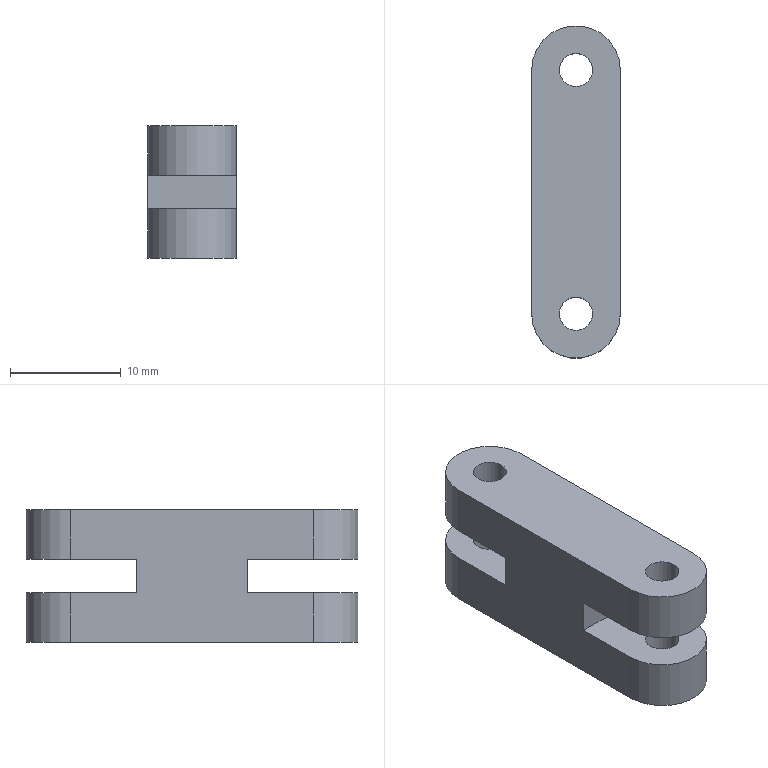Part | SolidWorks | features ICE 2, 3DProfileFeature 1, Extrusion 1, HoleWzd 1 | 1 solid | 26 faces | box 8 x 30 x 12 mm | volume 2022 mm3 | cylinder 14 | plane 10 | cone 2 | commonest cylinder face diameters 3 x8 8 x4 5 x2
STEP:
#1=CARTESIAN_POINT('',(-2.,11.,8.5));
#2=VERTEX_POINT('',#1);
#3=CARTESIAN_POINT('',(-2.,11.,3.5));
#4=VERTEX_POINT('',#3);
#5=CARTESIAN_POINT('',(-2.,11.,6.));
#6=DIRECTION('',(1.,0.,0.));
#7=DIRECTION('',(0.,0.,-1.));
#8=AXIS2_PLACEMENT_3D('',#5,#6,#7);
#9=CIRCLE('',#8,2.5);
#10=EDGE_CURVE('',#2,#4,#9,.T.);
#11=ORIENTED_EDGE('',*,*,#10,.F.);
#12=CARTESIAN_POINT('',(4.,11.,8.5));
#13=VERTEX_POINT('',#12);
#14=CARTESIAN_POINT('',(4.,11.,8.5));
#15=DIRECTION('',(1.,0.,0.));
#16=VECTOR('',#15,1000.);
#17=LINE('',#14,#16);
#18=EDGE_CURVE('',#2,#13,#17,.T.);
#19=ORIENTED_EDGE('',*,*,#18,.T.);
#20=CARTESIAN_POINT('',(4.,11.,3.5));
#21=VERTEX_POINT('',#20);
#22=CARTESIAN_POINT('',(4.,11.,6.));
#23=DIRECTION('',(1.,0.,0.));
#24=DIRECTION('',(0.,0.,-1.));
#25=AXIS2_PLACEMENT_3D('',#22,#23,#24);
#26=CIRCLE('',#25,2.5);
#27=EDGE_CURVE('',#13,#21,#26,.T.);
#28=ORIENTED_EDGE('',*,*,#27,.T.);
#29=CARTESIAN_POINT('',(4.,11.,3.5));
#30=DIRECTION('',(1.,0.,0.));
#31=VECTOR('',#30,1000.);
#32=LINE('',#29,#31);
#33=EDGE_CURVE('',#4,#21,#32,.T.);
#34=ORIENTED_EDGE('',*,*,#33,.F.);
#35=EDGE_LOOP('',(#11,#19,#28,#34));
#36=FACE_OUTER_BOUND('',#35,.T.);
#37=CARTESIAN_POINT('',(4.,11.,6.));
#38=DIRECTION('',(1.,0.,0.));
#39=DIRECTION('',(0.,0.,-1.));
#40=AXIS2_PLACEMENT_3D('',#37,#38,#39);
#41=CYLINDRICAL_SURFACE('',#40,2.5);
#42=ADVANCED_FACE('',(#36),#41,.F.);
#43=CARTESIAN_POINT('',(-3.502,11.,6.));
#44=VERTEX_POINT('',#43);
#45=CARTESIAN_POINT('',(-2.,11.,3.5));
#46=DIRECTION('',(0.515,0.,-0.8572));
#47=VECTOR('',#46,1000.);
#48=LINE('',#45,#47);
#49=EDGE_CURVE('',#44,#4,#48,.T.);
#50=ORIENTED_EDGE('',*,*,#49,.F.);
#51=CARTESIAN_POINT('',(-2.,11.,8.5));
#52=DIRECTION('',(0.515,0.,0.8572));
#53=VECTOR('',#52,1000.);
#54=LINE('',#51,#53);
#55=EDGE_CURVE('',#44,#2,#54,.T.);
#56=ORIENTED_EDGE('',*,*,#55,.T.);
#57=ORIENTED_EDGE('',*,*,#10,.T.);
#58=EDGE_LOOP('',(#50,#56,#57));
#59=FACE_OUTER_BOUND('',#58,.T.);
#60=CARTESIAN_POINT('',(-2.,11.,6.));
#61=DIRECTION('',(1.,0.,0.));
#62=DIRECTION('',(0.,0.,-1.));
#63=AXIS2_PLACEMENT_3D('',#60,#61,#62);
#64=CONICAL_SURFACE('',#63,2.5,1.03);
#65=ADVANCED_FACE('',(#59),#64,.F.);
#66=CARTESIAN_POINT('',(-1.5,0.,0.));
#67=VERTEX_POINT('',#66);
#68=CARTESIAN_POINT('',(1.5,0.,0.));
#69=VERTEX_POINT('',#68);
#70=CARTESIAN_POINT('',(0.,0.,0.));
#71=DIRECTION('',(0.,0.,1.));
#72=DIRECTION('',(1.,0.,0.));
#73=AXIS2_PLACEMENT_3D('',#70,#71,#72);
#74=CIRCLE('',#73,1.5);
#75=EDGE_CURVE('',#67,#69,#74,.T.);
#76=ORIENTED_EDGE('',*,*,#75,.F.);
#77=CARTESIAN_POINT('',(-1.5,0.,4.5));
#78=VERTEX_POINT('',#77);
#79=CARTESIAN_POINT('',(-1.5,0.,0.));
#80=DIRECTION('',(0.,0.,1.));
#81=VECTOR('',#80,1000.);
#82=LINE('',#79,#81);
#83=EDGE_CURVE('',#67,#78,#82,.T.);
#84=ORIENTED_EDGE('',*,*,#83,.T.);
#85=CARTESIAN_POINT('',(1.5,0.,4.5));
#86=VERTEX_POINT('',#85);
#87=CARTESIAN_POINT('',(0.,0.,4.5));
#88=DIRECTION('',(0.,0.,-1.));
#89=DIRECTION('',(-1.,0.,0.));
#90=AXIS2_PLACEMENT_3D('',#87,#88,#89);
#91=CIRCLE('',#90,1.5);
#92=EDGE_CURVE('',#86,#78,#91,.T.);
#93=ORIENTED_EDGE('',*,*,#92,.F.);
#94=CARTESIAN_POINT('',(1.5,0.,0.));
#95=DIRECTION('',(0.,0.,1.));
#96=VECTOR('',#95,1000.);
#97=LINE('',#94,#96);
#98=EDGE_CURVE('',#69,#86,#97,.T.);
#99=ORIENTED_EDGE('',*,*,#98,.F.);
#100=EDGE_LOOP('',(#76,#84,#93,#99));
#101=FACE_OUTER_BOUND('',#100,.T.);
#102=CARTESIAN_POINT('',(0.,0.,0.));
#103=DIRECTION('',(0.,0.,1.));
#104=DIRECTION('',(1.,0.,0.));
#105=AXIS2_PLACEMENT_3D('',#102,#103,#104);
#106=CYLINDRICAL_SURFACE('',#105,1.5);
#107=ADVANCED_FACE('',(#101),#106,.F.);
#108=CARTESIAN_POINT('',(-1.5,0.,7.5));
#109=VERTEX_POINT('',#108);
#110=CARTESIAN_POINT('',(1.5,0.,7.5));
#111=VERTEX_POINT('',#110);
#112=CARTESIAN_POINT('',(0.,0.,7.5));
#113=DIRECTION('',(0.,0.,1.));
#114=DIRECTION('',(0.,-1.,0.));
#115=AXIS2_PLACEMENT_3D('',#112,#113,#114);
#116=CIRCLE('',#115,1.5);
#117=EDGE_CURVE('',#109,#111,#116,.T.);
#118=ORIENTED_EDGE('',*,*,#117,.F.);
#119=CARTESIAN_POINT('',(-1.5,0.,12.));
#120=VERTEX_POINT('',#119);
#121=CARTESIAN_POINT('',(-1.5,0.,0.));
#122=DIRECTION('',(0.,0.,1.));
#123=VECTOR('',#122,1000.);
#124=LINE('',#121,#123);
#125=EDGE_CURVE('',#109,#120,#124,.T.);
#126=ORIENTED_EDGE('',*,*,#125,.T.);
#127=CARTESIAN_POINT('',(1.5,0.,12.));
#128=VERTEX_POINT('',#127);
#129=CARTESIAN_POINT('',(0.,0.,12.));
#130=DIRECTION('',(0.,0.,1.));
#131=DIRECTION('',(1.,0.,0.));
#132=AXIS2_PLACEMENT_3D('',#129,#130,#131);
#133=CIRCLE('',#132,1.5);
#134=EDGE_CURVE('',#120,#128,#133,.T.);
#135=ORIENTED_EDGE('',*,*,#134,.T.);
#136=CARTESIAN_POINT('',(1.5,0.,0.));
#137=DIRECTION('',(0.,0.,1.));
#138=VECTOR('',#137,1000.);
#139=LINE('',#136,#138);
#140=EDGE_CURVE('',#111,#128,#139,.T.);
#141=ORIENTED_EDGE('',*,*,#140,.F.);
#142=EDGE_LOOP('',(#118,#126,#135,#141));
#143=FACE_OUTER_BOUND('',#142,.T.);
#144=CARTESIAN_POINT('',(0.,0.,0.));
#145=DIRECTION('',(0.,0.,1.));
#146=DIRECTION('',(1.,0.,0.));
#147=AXIS2_PLACEMENT_3D('',#144,#145,#146);
#148=CYLINDRICAL_SURFACE('',#147,1.5);
#149=ADVANCED_FACE('',(#143),#148,.F.);
#150=CARTESIAN_POINT('',(-1.5,22.,7.5));
#151=VERTEX_POINT('',#150);
#152=CARTESIAN_POINT('',(1.5,22.,7.5));
#153=VERTEX_POINT('',#152);
#154=CARTESIAN_POINT('',(0.,22.,7.5));
#155=DIRECTION('',(0.,0.,1.));
#156=DIRECTION('',(0.,-1.,0.));
#157=AXIS2_PLACEMENT_3D('',#154,#155,#156);
#158=CIRCLE('',#157,1.5);
#159=EDGE_CURVE('',#151,#153,#158,.T.);
#160=ORIENTED_EDGE('',*,*,#159,.F.);
#161=CARTESIAN_POINT('',(-1.5,22.,12.));
#162=VERTEX_POINT('',#161);
#163=CARTESIAN_POINT('',(-1.5,22.,0.));
#164=DIRECTION('',(0.,0.,1.));
#165=VECTOR('',#164,1000.);
#166=LINE('',#163,#165);
#167=EDGE_CURVE('',#151,#162,#166,.T.);
#168=ORIENTED_EDGE('',*,*,#167,.T.);
#169=CARTESIAN_POINT('',(1.5,22.,12.));
#170=VERTEX_POINT('',#169);
#171=CARTESIAN_POINT('',(0.,22.,12.));
#172=DIRECTION('',(0.,0.,1.));
#173=DIRECTION('',(1.,0.,0.));
#174=AXIS2_PLACEMENT_3D('',#171,#172,#173);
#175=CIRCLE('',#174,1.5);
#176=EDGE_CURVE('',#162,#170,#175,.T.);
#177=ORIENTED_EDGE('',*,*,#176,.T.);
#178=CARTESIAN_POINT('',(1.5,22.,0.));
#179=DIRECTION('',(0.,0.,1.));
#180=VECTOR('',#179,1000.);
#181=LINE('',#178,#180);
#182=EDGE_CURVE('',#153,#170,#181,.T.);
#183=ORIENTED_EDGE('',*,*,#182,.F.);
#184=EDGE_LOOP('',(#160,#168,#177,#183));
#185=FACE_OUTER_BOUND('',#184,.T.);
#186=CARTESIAN_POINT('',(0.,22.,0.));
#187=DIRECTION('',(0.,0.,1.));
#188=DIRECTION('',(1.,0.,0.));
#189=AXIS2_PLACEMENT_3D('',#186,#187,#188);
#190=CYLINDRICAL_SURFACE('',#189,1.5);
#191=ADVANCED_FACE('',(#185),#190,.F.);
#192=CARTESIAN_POINT('',(-1.5,22.,0.));
#193=VERTEX_POINT('',#192);
#194=CARTESIAN_POINT('',(1.5,22.,0.));
#195=VERTEX_POINT('',#194);
#196=CARTESIAN_POINT('',(0.,22.,0.));
#197=DIRECTION('',(0.,0.,1.));
#198=DIRECTION('',(1.,0.,0.));
#199=AXIS2_PLACEMENT_3D('',#196,#197,#198);
#200=CIRCLE('',#199,1.5);
#201=EDGE_CURVE('',#193,#195,#200,.T.);
#202=ORIENTED_EDGE('',*,*,#201,.F.);
#203=CARTESIAN_POINT('',(-1.5,22.,4.5));
#204=VERTEX_POINT('',#203);
#205=CARTESIAN_POINT('',(-1.5,22.,0.));
#206=DIRECTION('',(0.,0.,1.));
#207=VECTOR('',#206,1000.);
#208=LINE('',#205,#207);
#209=EDGE_CURVE('',#193,#204,#208,.T.);
#210=ORIENTED_EDGE('',*,*,#209,.T.);
#211=CARTESIAN_POINT('',(1.5,22.,4.5));
#212=VERTEX_POINT('',#211);
#213=CARTESIAN_POINT('',(0.,22.,4.5));
#214=DIRECTION('',(0.,0.,-1.));
#215=DIRECTION('',(-1.,0.,0.));
#216=AXIS2_PLACEMENT_3D('',#213,#214,#215);
#217=CIRCLE('',#216,1.5);
#218=EDGE_CURVE('',#212,#204,#217,.T.);
#219=ORIENTED_EDGE('',*,*,#218,.F.);
#220=CARTESIAN_POINT('',(1.5,22.,0.));
#221=DIRECTION('',(0.,0.,1.));
#222=VECTOR('',#221,1000.);
#223=LINE('',#220,#222);
#224=EDGE_CURVE('',#195,#212,#223,.T.);
#225=ORIENTED_EDGE('',*,*,#224,.F.);
#226=EDGE_LOOP('',(#202,#210,#219,#225));
#227=FACE_OUTER_BOUND('',#226,.T.);
#228=CARTESIAN_POINT('',(0.,22.,0.));
#229=DIRECTION('',(0.,0.,1.));
#230=DIRECTION('',(1.,0.,0.));
#231=AXIS2_PLACEMENT_3D('',#228,#229,#230);
#232=CYLINDRICAL_SURFACE('',#231,1.5);
#233=ADVANCED_FACE('',(#227),#232,.F.);
#234=CARTESIAN_POINT('',(4.,0.,4.5));
#235=VERTEX_POINT('',#234);
#236=CARTESIAN_POINT('',(4.,0.,0.));
#237=VERTEX_POINT('',#236);
#238=CARTESIAN_POINT('',(4.,0.,12.));
#239=DIRECTION('',(0.,0.,-1.));
#240=VECTOR('',#239,1000.);
#241=LINE('',#238,#240);
#242=EDGE_CURVE('',#235,#237,#241,.T.);
#243=ORIENTED_EDGE('',*,*,#242,.F.);
#244=CARTESIAN_POINT('',(-4.,0.,4.5));
#245=VERTEX_POINT('',#244);
#246=CARTESIAN_POINT('',(0.,0.,4.5));
#247=DIRECTION('',(0.,0.,-1.));
#248=DIRECTION('',(-1.,0.,0.));
#249=AXIS2_PLACEMENT_3D('',#246,#247,#248);
#250=CIRCLE('',#249,4.);
#251=EDGE_CURVE('',#235,#245,#250,.T.);
#252=ORIENTED_EDGE('',*,*,#251,.T.);
#253=CARTESIAN_POINT('',(-4.,0.,0.));
#254=VERTEX_POINT('',#253);
#255=CARTESIAN_POINT('',(-4.,0.,12.));
#256=DIRECTION('',(0.,0.,-1.));
#257=VECTOR('',#256,1000.);
#258=LINE('',#255,#257);
#259=EDGE_CURVE('',#245,#254,#258,.T.);
#260=ORIENTED_EDGE('',*,*,#259,.T.);
#261=CARTESIAN_POINT('',(0.,0.,0.));
#262=DIRECTION('',(0.,0.,1.));
#263=DIRECTION('',(1.,0.,0.));
#264=AXIS2_PLACEMENT_3D('',#261,#262,#263);
#265=CIRCLE('',#264,4.);
#266=EDGE_CURVE('',#254,#237,#265,.T.);
#267=ORIENTED_EDGE('',*,*,#266,.T.);
#268=EDGE_LOOP('',(#243,#252,#260,#267));
#269=FACE_OUTER_BOUND('',#268,.T.);
#270=CARTESIAN_POINT('',(0.,0.,12.));
#271=DIRECTION('',(0.,0.,-1.));
#272=DIRECTION('',(-1.,0.,0.));
#273=AXIS2_PLACEMENT_3D('',#270,#271,#272);
#274=CYLINDRICAL_SURFACE('',#273,4.);
#275=ADVANCED_FACE('',(#269),#274,.T.);
#276=CARTESIAN_POINT('',(4.,22.,12.));
#277=VERTEX_POINT('',#276);
#278=CARTESIAN_POINT('',(4.,22.,7.5));
#279=VERTEX_POINT('',#278);
#280=CARTESIAN_POINT('',(4.,22.,12.));
#281=DIRECTION('',(0.,0.,-1.));
#282=VECTOR('',#281,1000.);
#283=LINE('',#280,#282);
#284=EDGE_CURVE('',#277,#279,#283,.T.);
#285=ORIENTED_EDGE('',*,*,#284,.T.);
#286=CARTESIAN_POINT('',(-4.,22.,7.5));
#287=VERTEX_POINT('',#286);
#288=CARTESIAN_POINT('',(0.,22.,7.5));
#289=DIRECTION('',(0.,0.,1.));
#290=DIRECTION('',(0.,-1.,0.));
#291=AXIS2_PLACEMENT_3D('',#288,#289,#290);
#292=CIRCLE('',#291,4.);
#293=EDGE_CURVE('',#279,#287,#292,.T.);
#294=ORIENTED_EDGE('',*,*,#293,.T.);
#295=CARTESIAN_POINT('',(-4.,22.,12.));
#296=VERTEX_POINT('',#295);
#297=CARTESIAN_POINT('',(-4.,22.,12.));
#298=DIRECTION('',(0.,0.,-1.));
#299=VECTOR('',#298,1000.);
#300=LINE('',#297,#299);
#301=EDGE_CURVE('',#296,#287,#300,.T.);
#302=ORIENTED_EDGE('',*,*,#301,.F.);
#303=CARTESIAN_POINT('',(0.,22.,12.));
#304=DIRECTION('',(0.,0.,1.));
#305=DIRECTION('',(1.,0.,0.));
#306=AXIS2_PLACEMENT_3D('',#303,#304,#305);
#307=CIRCLE('',#306,4.);
#308=EDGE_CURVE('',#277,#296,#307,.T.);
#309=ORIENTED_EDGE('',*,*,#308,.F.);
#310=EDGE_LOOP('',(#285,#294,#302,#309));
#311=FACE_OUTER_BOUND('',#310,.T.);
#312=CARTESIAN_POINT('',(0.,22.,12.));
#313=DIRECTION('',(0.,0.,-1.));
#314=DIRECTION('',(-1.,0.,0.));
#315=AXIS2_PLACEMENT_3D('',#312,#313,#314);
#316=CYLINDRICAL_SURFACE('',#315,4.);
#317=ADVANCED_FACE('',(#311),#316,.T.);
#318=CARTESIAN_POINT('',(-4.,0.,12.));
#319=VERTEX_POINT('',#318);
#320=CARTESIAN_POINT('',(-4.,0.,7.5));
#321=VERTEX_POINT('',#320);
#322=CARTESIAN_POINT('',(-4.,0.,12.));
#323=DIRECTION('',(0.,0.,-1.));
#324=VECTOR('',#323,1000.);
#325=LINE('',#322,#324);
#326=EDGE_CURVE('',#319,#321,#325,.T.);
#327=ORIENTED_EDGE('',*,*,#326,.T.);
#328=CARTESIAN_POINT('',(4.,0.,7.5));
#329=VERTEX_POINT('',#328);
#330=CARTESIAN_POINT('',(0.,0.,7.5));
#331=DIRECTION('',(0.,0.,1.));
#332=DIRECTION('',(0.,-1.,0.));
#333=AXIS2_PLACEMENT_3D('',#330,#331,#332);
#334=CIRCLE('',#333,4.);
#335=EDGE_CURVE('',#321,#329,#334,.T.);
#336=ORIENTED_EDGE('',*,*,#335,.T.);
#337=CARTESIAN_POINT('',(4.,0.,12.));
#338=VERTEX_POINT('',#337);
#339=CARTESIAN_POINT('',(4.,0.,12.));
#340=DIRECTION('',(0.,0.,-1.));
#341=VECTOR('',#340,1000.);
#342=LINE('',#339,#341);
#343=EDGE_CURVE('',#338,#329,#342,.T.);
#344=ORIENTED_EDGE('',*,*,#343,.F.);
#345=CARTESIAN_POINT('',(0.,0.,12.));
#346=DIRECTION('',(0.,0.,1.));
#347=DIRECTION('',(1.,0.,0.));
#348=AXIS2_PLACEMENT_3D('',#345,#346,#347);
#349=CIRCLE('',#348,4.);
#350=EDGE_CURVE('',#319,#338,#349,.T.);
#351=ORIENTED_EDGE('',*,*,#350,.F.);
#352=EDGE_LOOP('',(#327,#336,#344,#351));
#353=FACE_OUTER_BOUND('',#352,.T.);
#354=CARTESIAN_POINT('',(0.,0.,12.));
#355=DIRECTION('',(0.,0.,-1.));
#356=DIRECTION('',(-1.,0.,0.));
#357=AXIS2_PLACEMENT_3D('',#354,#355,#356);
#358=CYLINDRICAL_SURFACE('',#357,4.);
#359=ADVANCED_FACE('',(#353),#358,.T.);
#360=CARTESIAN_POINT('',(4.,11.,6.));
#361=DIRECTION('',(1.,0.,0.));
#362=DIRECTION('',(0.,0.,-1.));
#363=AXIS2_PLACEMENT_3D('',#360,#361,#362);
#364=CIRCLE('',#363,2.5);
#365=EDGE_CURVE('',#21,#13,#364,.T.);
#366=ORIENTED_EDGE('',*,*,#365,.F.);
#367=ORIENTED_EDGE('',*,*,#27,.F.);
#368=EDGE_LOOP('',(#366,#367));
#369=FACE_BOUND('',#368,.T.);
#370=CARTESIAN_POINT('',(4.,16.,4.5));
#371=VERTEX_POINT('',#370);
#372=CARTESIAN_POINT('',(4.,16.,7.5));
#373=VERTEX_POINT('',#372);
#374=CARTESIAN_POINT('',(4.,16.,4.5));
#375=DIRECTION('',(0.,0.,1.));
#376=VECTOR('',#375,1000.);
#377=LINE('',#374,#376);
#378=EDGE_CURVE('',#371,#373,#377,.T.);
#379=ORIENTED_EDGE('',*,*,#378,.T.);
#380=CARTESIAN_POINT('',(4.,36.,7.5));
#381=DIRECTION('',(0.,1.,0.));
#382=VECTOR('',#381,1000.);
#383=LINE('',#380,#382);
#384=EDGE_CURVE('',#373,#279,#383,.T.);
#385=ORIENTED_EDGE('',*,*,#384,.T.);
#386=ORIENTED_EDGE('',*,*,#284,.F.);
#387=CARTESIAN_POINT('',(4.,0.,12.));
#388=DIRECTION('',(0.,1.,0.));
#389=VECTOR('',#388,1000.);
#390=LINE('',#387,#389);
#391=EDGE_CURVE('',#338,#277,#390,.T.);
#392=ORIENTED_EDGE('',*,*,#391,.F.);
#393=ORIENTED_EDGE('',*,*,#343,.T.);
#394=CARTESIAN_POINT('',(4.,6.,7.5));
#395=VERTEX_POINT('',#394);
#396=CARTESIAN_POINT('',(4.,-14.,7.5));
#397=DIRECTION('',(0.,1.,0.));
#398=VECTOR('',#397,1000.);
#399=LINE('',#396,#398);
#400=EDGE_CURVE('',#329,#395,#399,.T.);
#401=ORIENTED_EDGE('',*,*,#400,.T.);
#402=CARTESIAN_POINT('',(4.,6.,4.5));
#403=VERTEX_POINT('',#402);
#404=CARTESIAN_POINT('',(4.,6.,4.5));
#405=DIRECTION('',(0.,0.,-1.));
#406=VECTOR('',#405,1000.);
#407=LINE('',#404,#406);
#408=EDGE_CURVE('',#395,#403,#407,.T.);
#409=ORIENTED_EDGE('',*,*,#408,.T.);
#410=CARTESIAN_POINT('',(4.,-14.,4.5));
#411=DIRECTION('',(0.,-1.,0.));
#412=VECTOR('',#411,1000.);
#413=LINE('',#410,#412);
#414=EDGE_CURVE('',#403,#235,#413,.T.);
#415=ORIENTED_EDGE('',*,*,#414,.T.);
#416=ORIENTED_EDGE('',*,*,#242,.T.);
#417=CARTESIAN_POINT('',(4.,22.,0.));
#418=VERTEX_POINT('',#417);
#419=CARTESIAN_POINT('',(4.,0.,0.));
#420=DIRECTION('',(0.,1.,0.));
#421=VECTOR('',#420,1000.);
#422=LINE('',#419,#421);
#423=EDGE_CURVE('',#237,#418,#422,.T.);
#424=ORIENTED_EDGE('',*,*,#423,.T.);
#425=CARTESIAN_POINT('',(4.,22.,4.5));
#426=VERTEX_POINT('',#425);
#427=CARTESIAN_POINT('',(4.,22.,12.));
#428=DIRECTION('',(0.,0.,-1.));
#429=VECTOR('',#428,1000.);
#430=LINE('',#427,#429);
#431=EDGE_CURVE('',#426,#418,#430,.T.);
#432=ORIENTED_EDGE('',*,*,#431,.F.);
#433=CARTESIAN_POINT('',(4.,36.,4.5));
#434=DIRECTION('',(0.,-1.,0.));
#435=VECTOR('',#434,1000.);
#436=LINE('',#433,#435);
#437=EDGE_CURVE('',#426,#371,#436,.T.);
#438=ORIENTED_EDGE('',*,*,#437,.T.);
#439=EDGE_LOOP('',(#379,#385,#386,#392,#393,#401,#409,#415,#416,#424,#432,#438));
#440=FACE_OUTER_BOUND('',#439,.T.);
#441=CARTESIAN_POINT('',(4.,0.,12.));
#442=DIRECTION('',(-1.,0.,0.));
#443=DIRECTION('',(0.,0.,1.));
#444=AXIS2_PLACEMENT_3D('',#441,#442,#443);
#445=PLANE('',#444);
#446=ADVANCED_FACE('',(#369,#440),#445,.F.);
#447=CARTESIAN_POINT('',(-4.,22.,4.5));
#448=VERTEX_POINT('',#447);
#449=CARTESIAN_POINT('',(-4.,22.,0.));
#450=VERTEX_POINT('',#449);
#451=CARTESIAN_POINT('',(-4.,22.,12.));
#452=DIRECTION('',(0.,0.,-1.));
#453=VECTOR('',#452,1000.);
#454=LINE('',#451,#453);
#455=EDGE_CURVE('',#448,#450,#454,.T.);
#456=ORIENTED_EDGE('',*,*,#455,.F.);
#457=CARTESIAN_POINT('',(0.,22.,4.5));
#458=DIRECTION('',(0.,0.,-1.));
#459=DIRECTION('',(-1.,0.,0.));
#460=AXIS2_PLACEMENT_3D('',#457,#458,#459);
#461=CIRCLE('',#460,4.);
#462=EDGE_CURVE('',#448,#426,#461,.T.);
#463=ORIENTED_EDGE('',*,*,#462,.T.);
#464=ORIENTED_EDGE('',*,*,#431,.T.);
#465=CARTESIAN_POINT('',(0.,22.,0.));
#466=DIRECTION('',(0.,0.,1.));
#467=DIRECTION('',(1.,0.,0.));
#468=AXIS2_PLACEMENT_3D('',#465,#466,#467);
#469=CIRCLE('',#468,4.);
#470=EDGE_CURVE('',#418,#450,#469,.T.);
#471=ORIENTED_EDGE('',*,*,#470,.T.);
#472=EDGE_LOOP('',(#456,#463,#464,#471));
#473=FACE_OUTER_BOUND('',#472,.T.);
#474=CARTESIAN_POINT('',(0.,22.,12.));
#475=DIRECTION('',(0.,0.,-1.));
#476=DIRECTION('',(-1.,0.,0.));
#477=AXIS2_PLACEMENT_3D('',#474,#475,#476);
#478=CYLINDRICAL_SURFACE('',#477,4.);
#479=ADVANCED_FACE('',(#473),#478,.T.);
#480=ORIENTED_EDGE('',*,*,#301,.T.);
#481=CARTESIAN_POINT('',(-4.,16.,7.5));
#482=VERTEX_POINT('',#481);
#483=CARTESIAN_POINT('',(-4.,36.,7.5));
#484=DIRECTION('',(0.,1.,0.));
#485=VECTOR('',#484,1000.);
#486=LINE('',#483,#485);
#487=EDGE_CURVE('',#482,#287,#486,.T.);
#488=ORIENTED_EDGE('',*,*,#487,.F.);
#489=CARTESIAN_POINT('',(-4.,16.,4.5));
#490=VERTEX_POINT('',#489);
#491=CARTESIAN_POINT('',(-4.,16.,4.5));
#492=DIRECTION('',(0.,0.,1.));
#493=VECTOR('',#492,1000.);
#494=LINE('',#491,#493);
#495=EDGE_CURVE('',#490,#482,#494,.T.);
#496=ORIENTED_EDGE('',*,*,#495,.F.);
#497=CARTESIAN_POINT('',(-4.,0.,4.5));
#498=DIRECTION('',(0.,1.,0.));
#499=VECTOR('',#498,1000.);
#500=LINE('',#497,#499);
#501=EDGE_CURVE('',#490,#448,#500,.T.);
#502=ORIENTED_EDGE('',*,*,#501,.T.);
#503=ORIENTED_EDGE('',*,*,#455,.T.);
#504=CARTESIAN_POINT('',(-4.,0.,0.));
#505=DIRECTION('',(0.,-1.,0.));
#506=VECTOR('',#505,1000.);
#507=LINE('',#504,#506);
#508=EDGE_CURVE('',#450,#254,#507,.T.);
#509=ORIENTED_EDGE('',*,*,#508,.T.);
#510=ORIENTED_EDGE('',*,*,#259,.F.);
#511=CARTESIAN_POINT('',(-4.,6.,4.5));
#512=VERTEX_POINT('',#511);
#513=CARTESIAN_POINT('',(-4.,-14.,4.5));
#514=DIRECTION('',(0.,-1.,0.));
#515=VECTOR('',#514,1000.);
#516=LINE('',#513,#515);
#517=EDGE_CURVE('',#512,#245,#516,.T.);
#518=ORIENTED_EDGE('',*,*,#517,.F.);
#519=CARTESIAN_POINT('',(-4.,6.,7.5));
#520=VERTEX_POINT('',#519);
#521=CARTESIAN_POINT('',(-4.,6.,4.5));
#522=DIRECTION('',(0.,0.,-1.));
#523=VECTOR('',#522,1000.);
#524=LINE('',#521,#523);
#525=EDGE_CURVE('',#520,#512,#524,.T.);
#526=ORIENTED_EDGE('',*,*,#525,.F.);
#527=CARTESIAN_POINT('',(-4.,0.,7.5));
#528=DIRECTION('',(0.,-1.,0.));
#529=VECTOR('',#528,1000.);
#530=LINE('',#527,#529);
#531=EDGE_CURVE('',#520,#321,#530,.T.);
#532=ORIENTED_EDGE('',*,*,#531,.T.);
#533=ORIENTED_EDGE('',*,*,#326,.F.);
#534=CARTESIAN_POINT('',(-4.,0.,12.));
#535=DIRECTION('',(0.,-1.,0.));
#536=VECTOR('',#535,1000.);
#537=LINE('',#534,#536);
#538=EDGE_CURVE('',#296,#319,#537,.T.);
#539=ORIENTED_EDGE('',*,*,#538,.F.);
#540=EDGE_LOOP('',(#480,#488,#496,#502,#503,#509,#510,#518,#526,#532,#533,#539));
#541=FACE_OUTER_BOUND('',#540,.T.);
#542=CARTESIAN_POINT('',(-4.,0.,12.));
#543=DIRECTION('',(1.,0.,0.));
#544=DIRECTION('',(0.,0.,-1.));
#545=AXIS2_PLACEMENT_3D('',#542,#543,#544);
#546=PLANE('',#545);
#547=ADVANCED_FACE('',(#541),#546,.F.);
#548=CARTESIAN_POINT('',(0.,22.,12.));
#549=DIRECTION('',(0.,0.,1.));
#550=DIRECTION('',(1.,0.,0.));
#551=AXIS2_PLACEMENT_3D('',#548,#549,#550);
#552=CIRCLE('',#551,1.5);
#553=EDGE_CURVE('',#170,#162,#552,.T.);
#554=ORIENTED_EDGE('',*,*,#553,.F.);
#555=ORIENTED_EDGE('',*,*,#176,.F.);
#556=EDGE_LOOP('',(#554,#555));
#557=FACE_BOUND('',#556,.T.);
#558=CARTESIAN_POINT('',(0.,0.,12.));
#559=DIRECTION('',(0.,0.,1.));
#560=DIRECTION('',(1.,0.,0.));
#561=AXIS2_PLACEMENT_3D('',#558,#559,#560);
#562=CIRCLE('',#561,1.5);
#563=EDGE_CURVE('',#128,#120,#562,.T.);
#564=ORIENTED_EDGE('',*,*,#563,.F.);
#565=ORIENTED_EDGE('',*,*,#134,.F.);
#566=EDGE_LOOP('',(#564,#565));
#567=FACE_BOUND('',#566,.T.);
#568=ORIENTED_EDGE('',*,*,#350,.T.);
#569=ORIENTED_EDGE('',*,*,#391,.T.);
#570=ORIENTED_EDGE('',*,*,#308,.T.);
#571=ORIENTED_EDGE('',*,*,#538,.T.);
#572=EDGE_LOOP('',(#568,#569,#570,#571));
#573=FACE_OUTER_BOUND('',#572,.T.);
#574=CARTESIAN_POINT('',(0.,0.,12.));
#575=DIRECTION('',(0.,0.,1.));
#576=DIRECTION('',(1.,0.,0.));
#577=AXIS2_PLACEMENT_3D('',#574,#575,#576);
#578=PLANE('',#577);
#579=ADVANCED_FACE('',(#557,#567,#573),#578,.T.);
#580=CARTESIAN_POINT('',(0.,22.,0.));
#581=DIRECTION('',(0.,0.,1.));
#582=DIRECTION('',(1.,0.,0.));
#583=AXIS2_PLACEMENT_3D('',#580,#581,#582);
#584=CIRCLE('',#583,1.5);
#585=EDGE_CURVE('',#195,#193,#584,.T.);
#586=ORIENTED_EDGE('',*,*,#585,.T.);
#587=ORIENTED_EDGE('',*,*,#201,.T.);
#588=EDGE_LOOP('',(#586,#587));
#589=FACE_BOUND('',#588,.T.);
#590=CARTESIAN_POINT('',(0.,0.,0.));
#591=DIRECTION('',(0.,0.,1.));
#592=DIRECTION('',(1.,0.,0.));
#593=AXIS2_PLACEMENT_3D('',#590,#591,#592);
#594=CIRCLE('',#593,1.5);
#595=EDGE_CURVE('',#69,#67,#594,.T.);
#596=ORIENTED_EDGE('',*,*,#595,.T.);
#597=ORIENTED_EDGE('',*,*,#75,.T.);
#598=EDGE_LOOP('',(#596,#597));
#599=FACE_BOUND('',#598,.T.);
#600=ORIENTED_EDGE('',*,*,#266,.F.);
#601=ORIENTED_EDGE('',*,*,#508,.F.);
#602=ORIENTED_EDGE('',*,*,#470,.F.);
#603=ORIENTED_EDGE('',*,*,#423,.F.);
#604=EDGE_LOOP('',(#600,#601,#602,#603));
#605=FACE_OUTER_BOUND('',#604,.T.);
#606=CARTESIAN_POINT('',(0.,0.,0.));
#607=DIRECTION('',(0.,0.,1.));
#608=DIRECTION('',(1.,0.,0.));
#609=AXIS2_PLACEMENT_3D('',#606,#607,#608);
#610=PLANE('',#609);
#611=ADVANCED_FACE('',(#589,#599,#605),#610,.F.);
#612=ORIENTED_EDGE('',*,*,#92,.T.);
#613=CARTESIAN_POINT('',(0.,0.,4.5));
#614=DIRECTION('',(0.,0.,-1.));
#615=DIRECTION('',(-1.,0.,0.));
#616=AXIS2_PLACEMENT_3D('',#613,#614,#615);
#617=CIRCLE('',#616,1.5);
#618=EDGE_CURVE('',#78,#86,#617,.T.);
#619=ORIENTED_EDGE('',*,*,#618,.T.);
#620=EDGE_LOOP('',(#612,#619));
#621=FACE_BOUND('',#620,.T.);
#622=ORIENTED_EDGE('',*,*,#414,.F.);
#623=CARTESIAN_POINT('',(4.,6.,4.5));
#624=DIRECTION('',(-1.,0.,0.));
#625=VECTOR('',#624,1000.);
#626=LINE('',#623,#625);
#627=EDGE_CURVE('',#403,#512,#626,.T.);
#628=ORIENTED_EDGE('',*,*,#627,.T.);
#629=ORIENTED_EDGE('',*,*,#517,.T.);
#630=ORIENTED_EDGE('',*,*,#251,.F.);
#631=EDGE_LOOP('',(#622,#628,#629,#630));
#632=FACE_OUTER_BOUND('',#631,.T.);
#633=CARTESIAN_POINT('',(4.,-14.,4.5));
#634=DIRECTION('',(0.,0.,-1.));
#635=DIRECTION('',(-1.,0.,0.));
#636=AXIS2_PLACEMENT_3D('',#633,#634,#635);
#637=PLANE('',#636);
#638=ADVANCED_FACE('',(#621,#632),#637,.F.);
#639=CARTESIAN_POINT('',(0.,0.,7.5));
#640=DIRECTION('',(0.,0.,1.));
#641=DIRECTION('',(0.,-1.,0.));
#642=AXIS2_PLACEMENT_3D('',#639,#640,#641);
#643=CIRCLE('',#642,1.5);
#644=EDGE_CURVE('',#111,#109,#643,.T.);
#645=ORIENTED_EDGE('',*,*,#644,.T.);
#646=ORIENTED_EDGE('',*,*,#117,.T.);
#647=EDGE_LOOP('',(#645,#646));
#648=FACE_BOUND('',#647,.T.);
#649=ORIENTED_EDGE('',*,*,#531,.F.);
#650=CARTESIAN_POINT('',(4.,6.,7.5));
#651=DIRECTION('',(-1.,0.,0.));
#652=VECTOR('',#651,1000.);
#653=LINE('',#650,#652);
#654=EDGE_CURVE('',#395,#520,#653,.T.);
#655=ORIENTED_EDGE('',*,*,#654,.F.);
#656=ORIENTED_EDGE('',*,*,#400,.F.);
#657=ORIENTED_EDGE('',*,*,#335,.F.);
#658=EDGE_LOOP('',(#649,#655,#656,#657));
#659=FACE_OUTER_BOUND('',#658,.T.);
#660=CARTESIAN_POINT('',(4.,-14.,7.5));
#661=DIRECTION('',(0.,0.,1.));
#662=DIRECTION('',(0.,-1.,0.));
#663=AXIS2_PLACEMENT_3D('',#660,#661,#662);
#664=PLANE('',#663);
#665=ADVANCED_FACE('',(#648,#659),#664,.F.);
#666=ORIENTED_EDGE('',*,*,#525,.T.);
#667=ORIENTED_EDGE('',*,*,#627,.F.);
#668=ORIENTED_EDGE('',*,*,#408,.F.);
#669=ORIENTED_EDGE('',*,*,#654,.T.);
#670=EDGE_LOOP('',(#666,#667,#668,#669));
#671=FACE_OUTER_BOUND('',#670,.T.);
#672=CARTESIAN_POINT('',(4.,6.,4.5));
#673=DIRECTION('',(0.,1.,0.));
#674=DIRECTION('',(-1.,0.,0.));
#675=AXIS2_PLACEMENT_3D('',#672,#673,#674);
#676=PLANE('',#675);
#677=ADVANCED_FACE('',(#671),#676,.F.);
#678=CARTESIAN_POINT('',(0.,22.,7.5));
#679=DIRECTION('',(0.,0.,1.));
#680=DIRECTION('',(0.,-1.,0.));
#681=AXIS2_PLACEMENT_3D('',#678,#679,#680);
#682=CIRCLE('',#681,1.5);
#683=EDGE_CURVE('',#153,#151,#682,.T.);
#684=ORIENTED_EDGE('',*,*,#683,.T.);
#685=ORIENTED_EDGE('',*,*,#159,.T.);
#686=EDGE_LOOP('',(#684,#685));
#687=FACE_BOUND('',#686,.T.);
#688=ORIENTED_EDGE('',*,*,#384,.F.);
#689=CARTESIAN_POINT('',(4.,16.,7.5));
#690=DIRECTION('',(-1.,0.,0.));
#691=VECTOR('',#690,1000.);
#692=LINE('',#689,#691);
#693=EDGE_CURVE('',#373,#482,#692,.T.);
#694=ORIENTED_EDGE('',*,*,#693,.T.);
#695=ORIENTED_EDGE('',*,*,#487,.T.);
#696=ORIENTED_EDGE('',*,*,#293,.F.);
#697=EDGE_LOOP('',(#688,#694,#695,#696));
#698=FACE_OUTER_BOUND('',#697,.T.);
#699=CARTESIAN_POINT('',(4.,36.,7.5));
#700=DIRECTION('',(0.,0.,1.));
#701=DIRECTION('',(0.,-1.,0.));
#702=AXIS2_PLACEMENT_3D('',#699,#700,#701);
#703=PLANE('',#702);
#704=ADVANCED_FACE('',(#687,#698),#703,.F.);
#705=ORIENTED_EDGE('',*,*,#218,.T.);
#706=CARTESIAN_POINT('',(0.,22.,4.5));
#707=DIRECTION('',(0.,0.,-1.));
#708=DIRECTION('',(-1.,0.,0.));
#709=AXIS2_PLACEMENT_3D('',#706,#707,#708);
#710=CIRCLE('',#709,1.5);
#711=EDGE_CURVE('',#204,#212,#710,.T.);
#712=ORIENTED_EDGE('',*,*,#711,.T.);
#713=EDGE_LOOP('',(#705,#712));
#714=FACE_BOUND('',#713,.T.);
#715=ORIENTED_EDGE('',*,*,#501,.F.);
#716=CARTESIAN_POINT('',(4.,16.,4.5));
#717=DIRECTION('',(-1.,0.,0.));
#718=VECTOR('',#717,1000.);
#719=LINE('',#716,#718);
#720=EDGE_CURVE('',#371,#490,#719,.T.);
#721=ORIENTED_EDGE('',*,*,#720,.F.);
#722=ORIENTED_EDGE('',*,*,#437,.F.);
#723=ORIENTED_EDGE('',*,*,#462,.F.);
#724=EDGE_LOOP('',(#715,#721,#722,#723));
#725=FACE_OUTER_BOUND('',#724,.T.);
#726=CARTESIAN_POINT('',(4.,36.,4.5));
#727=DIRECTION('',(0.,0.,-1.));
#728=DIRECTION('',(-1.,0.,0.));
#729=AXIS2_PLACEMENT_3D('',#726,#727,#728);
#730=PLANE('',#729);
#731=ADVANCED_FACE('',(#714,#725),#730,.F.);
#732=ORIENTED_EDGE('',*,*,#495,.T.);
#733=ORIENTED_EDGE('',*,*,#693,.F.);
#734=ORIENTED_EDGE('',*,*,#378,.F.);
#735=ORIENTED_EDGE('',*,*,#720,.T.);
#736=EDGE_LOOP('',(#732,#733,#734,#735));
#737=FACE_OUTER_BOUND('',#736,.T.);
#738=CARTESIAN_POINT('',(4.,16.,4.5));
#739=DIRECTION('',(0.,-1.,0.));
#740=DIRECTION('',(1.,0.,0.));
#741=AXIS2_PLACEMENT_3D('',#738,#739,#740);
#742=PLANE('',#741);
#743=ADVANCED_FACE('',(#737),#742,.F.);
#744=ORIENTED_EDGE('',*,*,#209,.F.);
#745=ORIENTED_EDGE('',*,*,#585,.F.);
#746=ORIENTED_EDGE('',*,*,#224,.T.);
#747=ORIENTED_EDGE('',*,*,#711,.F.);
#748=EDGE_LOOP('',(#744,#745,#746,#747));
#749=FACE_OUTER_BOUND('',#748,.T.);
#750=CARTESIAN_POINT('',(0.,22.,0.));
#751=DIRECTION('',(0.,0.,1.));
#752=DIRECTION('',(1.,0.,0.));
#753=AXIS2_PLACEMENT_3D('',#750,#751,#752);
#754=CYLINDRICAL_SURFACE('',#753,1.5);
#755=ADVANCED_FACE('',(#749),#754,.F.);
#756=ORIENTED_EDGE('',*,*,#167,.F.);
#757=ORIENTED_EDGE('',*,*,#683,.F.);
#758=ORIENTED_EDGE('',*,*,#182,.T.);
#759=ORIENTED_EDGE('',*,*,#553,.T.);
#760=EDGE_LOOP('',(#756,#757,#758,#759));
#761=FACE_OUTER_BOUND('',#760,.T.);
#762=CARTESIAN_POINT('',(0.,22.,0.));
#763=DIRECTION('',(0.,0.,1.));
#764=DIRECTION('',(1.,0.,0.));
#765=AXIS2_PLACEMENT_3D('',#762,#763,#764);
#766=CYLINDRICAL_SURFACE('',#765,1.5);
#767=ADVANCED_FACE('',(#761),#766,.F.);
#768=ORIENTED_EDGE('',*,*,#125,.F.);
#769=ORIENTED_EDGE('',*,*,#644,.F.);
#770=ORIENTED_EDGE('',*,*,#140,.T.);
#771=ORIENTED_EDGE('',*,*,#563,.T.);
#772=EDGE_LOOP('',(#768,#769,#770,#771));
#773=FACE_OUTER_BOUND('',#772,.T.);
#774=CARTESIAN_POINT('',(0.,0.,0.));
#775=DIRECTION('',(0.,0.,1.));
#776=DIRECTION('',(1.,0.,0.));
#777=AXIS2_PLACEMENT_3D('',#774,#775,#776);
#778=CYLINDRICAL_SURFACE('',#777,1.5);
#779=ADVANCED_FACE('',(#773),#778,.F.);
#780=ORIENTED_EDGE('',*,*,#83,.F.);
#781=ORIENTED_EDGE('',*,*,#595,.F.);
#782=ORIENTED_EDGE('',*,*,#98,.T.);
#783=ORIENTED_EDGE('',*,*,#618,.F.);
#784=EDGE_LOOP('',(#780,#781,#782,#783));
#785=FACE_OUTER_BOUND('',#784,.T.);
#786=CARTESIAN_POINT('',(0.,0.,0.));
#787=DIRECTION('',(0.,0.,1.));
#788=DIRECTION('',(1.,0.,0.));
#789=AXIS2_PLACEMENT_3D('',#786,#787,#788);
#790=CYLINDRICAL_SURFACE('',#789,1.5);
#791=ADVANCED_FACE('',(#785),#790,.F.);
#792=ORIENTED_EDGE('',*,*,#55,.F.);
#793=ORIENTED_EDGE('',*,*,#49,.T.);
#794=CARTESIAN_POINT('',(-2.,11.,6.));
#795=DIRECTION('',(1.,0.,0.));
#796=DIRECTION('',(0.,0.,-1.));
#797=AXIS2_PLACEMENT_3D('',#794,#795,#796);
#798=CIRCLE('',#797,2.5);
#799=EDGE_CURVE('',#4,#2,#798,.T.);
#800=ORIENTED_EDGE('',*,*,#799,.T.);
#801=EDGE_LOOP('',(#792,#793,#800));
#802=FACE_OUTER_BOUND('',#801,.T.);
#803=CARTESIAN_POINT('',(-2.,11.,6.));
#804=DIRECTION('',(1.,0.,0.));
#805=DIRECTION('',(0.,0.,-1.));
#806=AXIS2_PLACEMENT_3D('',#803,#804,#805);
#807=CONICAL_SURFACE('',#806,2.5,1.03);
#808=ADVANCED_FACE('',(#802),#807,.F.);
#809=ORIENTED_EDGE('',*,*,#18,.F.);
#810=ORIENTED_EDGE('',*,*,#799,.F.);
#811=ORIENTED_EDGE('',*,*,#33,.T.);
#812=ORIENTED_EDGE('',*,*,#365,.T.);
#813=EDGE_LOOP('',(#809,#810,#811,#812));
#814=FACE_OUTER_BOUND('',#813,.T.);
#815=CARTESIAN_POINT('',(4.,11.,6.));
#816=DIRECTION('',(1.,0.,0.));
#817=DIRECTION('',(0.,0.,-1.));
#818=AXIS2_PLACEMENT_3D('',#815,#816,#817);
#819=CYLINDRICAL_SURFACE('',#818,2.5);
#820=ADVANCED_FACE('',(#814),#819,.F.);
#821=CLOSED_SHELL('',(#42,#65,#107,#149,#191,#233,#275,#317,#359,#446,#479,#547,#579,#611,#638,#665,#677,#704,#731,#743,#755,#767,#779,#791,#808,#820));
#822=MANIFOLD_SOLID_BREP('',#821);
#823=CARTESIAN_POINT('',(0.,0.,0.));
#824=DIRECTION('',(0.,0.,1.));
#825=DIRECTION('',(1.,0.,0.));
#826=AXIS2_PLACEMENT_3D('',#823,#824,#825);
#827=(LENGTH_UNIT()NAMED_UNIT(*)SI_UNIT(.MILLI.,.METRE.));
#828=UNCERTAINTY_MEASURE_WITH_UNIT(LENGTH_MEASURE(0.00001),#827,'','');
#829=(NAMED_UNIT(*)PLANE_ANGLE_UNIT()SI_UNIT($,.RADIAN.));
#830=(NAMED_UNIT(*)SI_UNIT($,.STERADIAN.)SOLID_ANGLE_UNIT());
#831=(GEOMETRIC_REPRESENTATION_CONTEXT(3)GLOBAL_UNCERTAINTY_ASSIGNED_CONTEXT((#828))GLOBAL_UNIT_ASSIGNED_CONTEXT((#827,#829,#830))REPRESENTATION_CONTEXT('',''));
#832=ADVANCED_BREP_SHAPE_REPRESENTATION('',(#822,#826),#831);